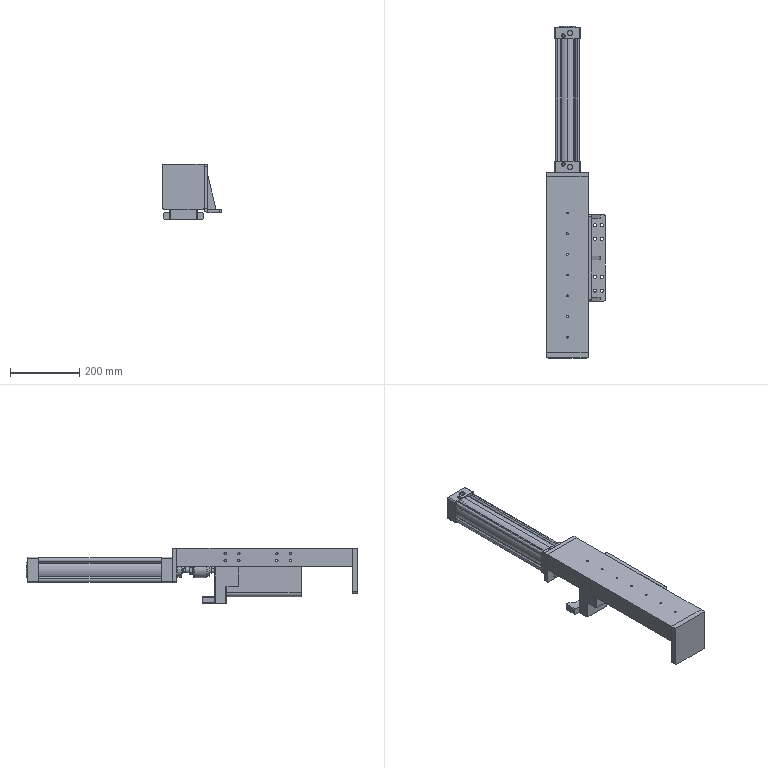Part | SolidWorks | 15 solids | 1033 faces | box 170 x 962 x 160 mm | volume 3347225 mm3 | plane 413 | cylinder 384 | cone 182 | spline 54 | commonest cylinder face diameters 9 x54 6.8 x50 12 x22 2.2 x18 11 x18 8.7 x16